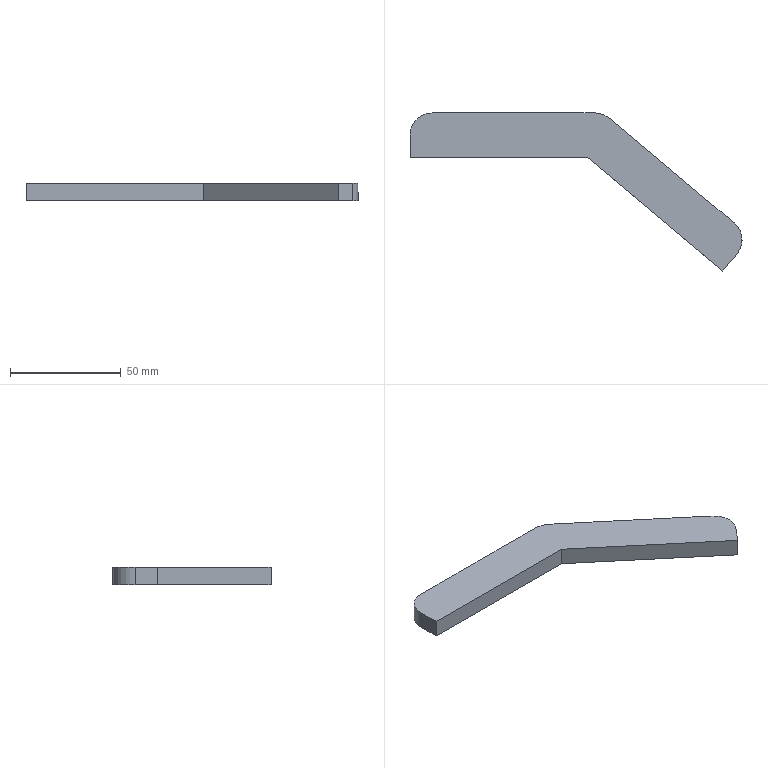Part | SolidWorks | features Extrusion 1, Fillet 1 | 1 solid | 11 faces | box 150.051 x 71.423 x 8 mm | volume 26409 mm3 | plane 8 | cylinder 3 | commonest cylinder face diameters 20 x3
STEP:
#1=CARTESIAN_POINT('',(0.,10.,8.));
#2=VERTEX_POINT('',#1);
#3=CARTESIAN_POINT('',(0.,0.,8.));
#4=VERTEX_POINT('',#3);
#5=CARTESIAN_POINT('',(0.,20.,8.));
#6=DIRECTION('',(0.,-1.,0.));
#7=VECTOR('',#6,1000.);
#8=LINE('',#5,#7);
#9=EDGE_CURVE('',#2,#4,#8,.T.);
#10=ORIENTED_EDGE('',*,*,#9,.F.);
#11=CARTESIAN_POINT('',(0.,10.,0.));
#12=VERTEX_POINT('',#11);
#13=CARTESIAN_POINT('',(0.,10.,8.));
#14=DIRECTION('',(0.,0.,-1.));
#15=VECTOR('',#14,1000.);
#16=LINE('',#13,#15);
#17=EDGE_CURVE('',#2,#12,#16,.T.);
#18=ORIENTED_EDGE('',*,*,#17,.T.);
#19=CARTESIAN_POINT('',(0.,0.,0.));
#20=VERTEX_POINT('',#19);
#21=CARTESIAN_POINT('',(0.,20.,0.));
#22=DIRECTION('',(0.,-1.,0.));
#23=VECTOR('',#22,1000.);
#24=LINE('',#21,#23);
#25=EDGE_CURVE('',#12,#20,#24,.T.);
#26=ORIENTED_EDGE('',*,*,#25,.T.);
#27=CARTESIAN_POINT('',(0.,0.,8.));
#28=DIRECTION('',(0.,0.,-1.));
#29=VECTOR('',#28,1000.);
#30=LINE('',#27,#29);
#31=EDGE_CURVE('',#4,#20,#30,.T.);
#32=ORIENTED_EDGE('',*,*,#31,.F.);
#33=EDGE_LOOP('',(#10,#18,#26,#32));
#34=FACE_OUTER_BOUND('',#33,.T.);
#35=CARTESIAN_POINT('',(0.,20.,8.));
#36=DIRECTION('',(1.,0.,0.));
#37=DIRECTION('',(0.,1.,0.));
#38=AXIS2_PLACEMENT_3D('',#35,#36,#37);
#39=PLANE('',#38);
#40=ADVANCED_FACE('',(#34),#39,.F.);
#41=CARTESIAN_POINT('',(80.,0.,0.));
#42=VERTEX_POINT('',#41);
#43=CARTESIAN_POINT('',(0.,0.,0.));
#44=DIRECTION('',(1.,0.,0.));
#45=VECTOR('',#44,1000.);
#46=LINE('',#43,#45);
#47=EDGE_CURVE('',#20,#42,#46,.T.);
#48=ORIENTED_EDGE('',*,*,#47,.T.);
#49=CARTESIAN_POINT('',(80.,0.,8.));
#50=VERTEX_POINT('',#49);
#51=CARTESIAN_POINT('',(80.,0.,8.));
#52=DIRECTION('',(0.,0.,-1.));
#53=VECTOR('',#52,1000.);
#54=LINE('',#51,#53);
#55=EDGE_CURVE('',#50,#42,#54,.T.);
#56=ORIENTED_EDGE('',*,*,#55,.F.);
#57=CARTESIAN_POINT('',(0.,0.,8.));
#58=DIRECTION('',(1.,0.,0.));
#59=VECTOR('',#58,1000.);
#60=LINE('',#57,#59);
#61=EDGE_CURVE('',#4,#50,#60,.T.);
#62=ORIENTED_EDGE('',*,*,#61,.F.);
#63=ORIENTED_EDGE('',*,*,#31,.T.);
#64=EDGE_LOOP('',(#48,#56,#62,#63));
#65=FACE_OUTER_BOUND('',#64,.T.);
#66=CARTESIAN_POINT('',(0.,0.,8.));
#67=DIRECTION('',(0.,1.,0.));
#68=DIRECTION('',(0.,0.,1.));
#69=AXIS2_PLACEMENT_3D('',#66,#67,#68);
#70=PLANE('',#69);
#71=ADVANCED_FACE('',(#65),#70,.F.);
#72=CARTESIAN_POINT('',(141.284,-51.423,0.));
#73=VERTEX_POINT('',#72);
#74=CARTESIAN_POINT('',(80.,0.,0.));
#75=DIRECTION('',(0.766,-0.6428,0.));
#76=VECTOR('',#75,1000.);
#77=LINE('',#74,#76);
#78=EDGE_CURVE('',#42,#73,#77,.T.);
#79=ORIENTED_EDGE('',*,*,#78,.T.);
#80=CARTESIAN_POINT('',(141.284,-51.423,8.));
#81=VERTEX_POINT('',#80);
#82=CARTESIAN_POINT('',(141.284,-51.423,8.));
#83=DIRECTION('',(0.,0.,-1.));
#84=VECTOR('',#83,1000.);
#85=LINE('',#82,#84);
#86=EDGE_CURVE('',#81,#73,#85,.T.);
#87=ORIENTED_EDGE('',*,*,#86,.F.);
#88=CARTESIAN_POINT('',(80.,0.,8.));
#89=DIRECTION('',(0.766,-0.6428,0.));
#90=VECTOR('',#89,1000.);
#91=LINE('',#88,#90);
#92=EDGE_CURVE('',#50,#81,#91,.T.);
#93=ORIENTED_EDGE('',*,*,#92,.F.);
#94=ORIENTED_EDGE('',*,*,#55,.T.);
#95=EDGE_LOOP('',(#79,#87,#93,#94));
#96=FACE_OUTER_BOUND('',#95,.T.);
#97=CARTESIAN_POINT('',(80.,0.,8.));
#98=DIRECTION('',(0.6428,0.766,0.));
#99=DIRECTION('',(-0.766,0.6428,0.));
#100=AXIS2_PLACEMENT_3D('',#97,#98,#99);
#101=PLANE('',#100);
#102=ADVANCED_FACE('',(#96),#101,.F.);
#103=CARTESIAN_POINT('',(147.711,-43.763,0.));
#104=VERTEX_POINT('',#103);
#105=CARTESIAN_POINT('',(141.284,-51.423,0.));
#106=DIRECTION('',(0.6428,0.766,0.));
#107=VECTOR('',#106,1000.);
#108=LINE('',#105,#107);
#109=EDGE_CURVE('',#73,#104,#108,.T.);
#110=ORIENTED_EDGE('',*,*,#109,.T.);
#111=CARTESIAN_POINT('',(147.711,-43.763,8.));
#112=VERTEX_POINT('',#111);
#113=CARTESIAN_POINT('',(147.711,-43.763,8.));
#114=DIRECTION('',(0.,0.,1.));
#115=VECTOR('',#114,1000.);
#116=LINE('',#113,#115);
#117=EDGE_CURVE('',#104,#112,#116,.T.);
#118=ORIENTED_EDGE('',*,*,#117,.T.);
#119=CARTESIAN_POINT('',(141.284,-51.423,8.));
#120=DIRECTION('',(0.6428,0.766,0.));
#121=VECTOR('',#120,1000.);
#122=LINE('',#119,#121);
#123=EDGE_CURVE('',#81,#112,#122,.T.);
#124=ORIENTED_EDGE('',*,*,#123,.F.);
#125=ORIENTED_EDGE('',*,*,#86,.T.);
#126=EDGE_LOOP('',(#110,#118,#124,#125));
#127=FACE_OUTER_BOUND('',#126,.T.);
#128=CARTESIAN_POINT('',(141.284,-51.423,8.));
#129=DIRECTION('',(-0.766,0.6428,0.));
#130=DIRECTION('',(-0.6428,-0.766,0.));
#131=AXIS2_PLACEMENT_3D('',#128,#129,#130);
#132=PLANE('',#131);
#133=ADVANCED_FACE('',(#127),#132,.F.);
#134=CARTESIAN_POINT('',(146.479,-29.674,0.));
#135=VERTEX_POINT('',#134);
#136=CARTESIAN_POINT('',(90.068,17.66,0.));
#137=VERTEX_POINT('',#136);
#138=CARTESIAN_POINT('',(154.139,-36.102,0.));
#139=DIRECTION('',(-0.766,0.6428,0.));
#140=VECTOR('',#139,1000.);
#141=LINE('',#138,#140);
#142=EDGE_CURVE('',#135,#137,#141,.T.);
#143=ORIENTED_EDGE('',*,*,#142,.T.);
#144=CARTESIAN_POINT('',(90.068,17.66,8.));
#145=VERTEX_POINT('',#144);
#146=CARTESIAN_POINT('',(90.068,17.66,8.));
#147=DIRECTION('',(0.,0.,1.));
#148=VECTOR('',#147,1000.);
#149=LINE('',#146,#148);
#150=EDGE_CURVE('',#137,#145,#149,.T.);
#151=ORIENTED_EDGE('',*,*,#150,.T.);
#152=CARTESIAN_POINT('',(146.479,-29.674,8.));
#153=VERTEX_POINT('',#152);
#154=CARTESIAN_POINT('',(154.139,-36.102,8.));
#155=DIRECTION('',(-0.766,0.6428,0.));
#156=VECTOR('',#155,1000.);
#157=LINE('',#154,#156);
#158=EDGE_CURVE('',#153,#145,#157,.T.);
#159=ORIENTED_EDGE('',*,*,#158,.F.);
#160=CARTESIAN_POINT('',(146.479,-29.674,8.));
#161=DIRECTION('',(0.,0.,-1.));
#162=VECTOR('',#161,1000.);
#163=LINE('',#160,#162);
#164=EDGE_CURVE('',#153,#135,#163,.T.);
#165=ORIENTED_EDGE('',*,*,#164,.T.);
#166=EDGE_LOOP('',(#143,#151,#159,#165));
#167=FACE_OUTER_BOUND('',#166,.T.);
#168=CARTESIAN_POINT('',(154.139,-36.102,8.));
#169=DIRECTION('',(-0.6428,-0.766,0.));
#170=DIRECTION('',(0.766,-0.6428,0.));
#171=AXIS2_PLACEMENT_3D('',#168,#169,#170);
#172=PLANE('',#171);
#173=ADVANCED_FACE('',(#167),#172,.F.);
#174=CARTESIAN_POINT('',(83.64,20.,8.));
#175=VERTEX_POINT('',#174);
#176=CARTESIAN_POINT('',(10.,20.,8.));
#177=VERTEX_POINT('',#176);
#178=CARTESIAN_POINT('',(87.279,20.,8.));
#179=DIRECTION('',(-1.,0.,0.));
#180=VECTOR('',#179,1000.);
#181=LINE('',#178,#180);
#182=EDGE_CURVE('',#175,#177,#181,.T.);
#183=ORIENTED_EDGE('',*,*,#182,.F.);
#184=CARTESIAN_POINT('',(83.64,20.,0.));
#185=VERTEX_POINT('',#184);
#186=CARTESIAN_POINT('',(83.64,20.,8.));
#187=DIRECTION('',(0.,0.,-1.));
#188=VECTOR('',#187,1000.);
#189=LINE('',#186,#188);
#190=EDGE_CURVE('',#175,#185,#189,.T.);
#191=ORIENTED_EDGE('',*,*,#190,.T.);
#192=CARTESIAN_POINT('',(10.,20.,0.));
#193=VERTEX_POINT('',#192);
#194=CARTESIAN_POINT('',(87.279,20.,0.));
#195=DIRECTION('',(-1.,0.,0.));
#196=VECTOR('',#195,1000.);
#197=LINE('',#194,#196);
#198=EDGE_CURVE('',#185,#193,#197,.T.);
#199=ORIENTED_EDGE('',*,*,#198,.T.);
#200=CARTESIAN_POINT('',(10.,20.,8.));
#201=DIRECTION('',(0.,0.,1.));
#202=VECTOR('',#201,1000.);
#203=LINE('',#200,#202);
#204=EDGE_CURVE('',#193,#177,#203,.T.);
#205=ORIENTED_EDGE('',*,*,#204,.T.);
#206=EDGE_LOOP('',(#183,#191,#199,#205));
#207=FACE_OUTER_BOUND('',#206,.T.);
#208=CARTESIAN_POINT('',(87.279,20.,8.));
#209=DIRECTION('',(0.,-1.,0.));
#210=DIRECTION('',(1.,0.,0.));
#211=AXIS2_PLACEMENT_3D('',#208,#209,#210);
#212=PLANE('',#211);
#213=ADVANCED_FACE('',(#207),#212,.F.);
#214=ORIENTED_EDGE('',*,*,#158,.T.);
#215=CARTESIAN_POINT('',(83.64,10.,8.));
#216=DIRECTION('',(0.,0.,1.));
#217=DIRECTION('',(1.,0.,0.));
#218=AXIS2_PLACEMENT_3D('',#215,#216,#217);
#219=CIRCLE('',#218,10.);
#220=EDGE_CURVE('',#145,#175,#219,.T.);
#221=ORIENTED_EDGE('',*,*,#220,.T.);
#222=ORIENTED_EDGE('',*,*,#182,.T.);
#223=CARTESIAN_POINT('',(10.,10.,8.));
#224=DIRECTION('',(0.,0.,1.));
#225=DIRECTION('',(1.,0.,0.));
#226=AXIS2_PLACEMENT_3D('',#223,#224,#225);
#227=CIRCLE('',#226,10.);
#228=EDGE_CURVE('',#177,#2,#227,.T.);
#229=ORIENTED_EDGE('',*,*,#228,.T.);
#230=ORIENTED_EDGE('',*,*,#9,.T.);
#231=ORIENTED_EDGE('',*,*,#61,.T.);
#232=ORIENTED_EDGE('',*,*,#92,.T.);
#233=ORIENTED_EDGE('',*,*,#123,.T.);
#234=CARTESIAN_POINT('',(140.051,-37.335,8.));
#235=DIRECTION('',(0.,0.,1.));
#236=DIRECTION('',(1.,0.,0.));
#237=AXIS2_PLACEMENT_3D('',#234,#235,#236);
#238=CIRCLE('',#237,10.);
#239=EDGE_CURVE('',#112,#153,#238,.T.);
#240=ORIENTED_EDGE('',*,*,#239,.T.);
#241=EDGE_LOOP('',(#214,#221,#222,#229,#230,#231,#232,#233,#240));
#242=FACE_OUTER_BOUND('',#241,.T.);
#243=CARTESIAN_POINT('',(0.,0.,8.));
#244=DIRECTION('',(0.,0.,1.));
#245=DIRECTION('',(1.,0.,0.));
#246=AXIS2_PLACEMENT_3D('',#243,#244,#245);
#247=PLANE('',#246);
#248=ADVANCED_FACE('',(#242),#247,.T.);
#249=ORIENTED_EDGE('',*,*,#198,.F.);
#250=CARTESIAN_POINT('',(83.64,10.,0.));
#251=DIRECTION('',(0.,0.,-1.));
#252=DIRECTION('',(1.,0.,0.));
#253=AXIS2_PLACEMENT_3D('',#250,#251,#252);
#254=CIRCLE('',#253,10.);
#255=EDGE_CURVE('',#185,#137,#254,.T.);
#256=ORIENTED_EDGE('',*,*,#255,.T.);
#257=ORIENTED_EDGE('',*,*,#142,.F.);
#258=CARTESIAN_POINT('',(140.051,-37.335,0.));
#259=DIRECTION('',(0.,0.,-1.));
#260=DIRECTION('',(1.,0.,0.));
#261=AXIS2_PLACEMENT_3D('',#258,#259,#260);
#262=CIRCLE('',#261,10.);
#263=EDGE_CURVE('',#135,#104,#262,.T.);
#264=ORIENTED_EDGE('',*,*,#263,.T.);
#265=ORIENTED_EDGE('',*,*,#109,.F.);
#266=ORIENTED_EDGE('',*,*,#78,.F.);
#267=ORIENTED_EDGE('',*,*,#47,.F.);
#268=ORIENTED_EDGE('',*,*,#25,.F.);
#269=CARTESIAN_POINT('',(10.,10.,0.));
#270=DIRECTION('',(0.,0.,-1.));
#271=DIRECTION('',(1.,0.,0.));
#272=AXIS2_PLACEMENT_3D('',#269,#270,#271);
#273=CIRCLE('',#272,10.);
#274=EDGE_CURVE('',#12,#193,#273,.T.);
#275=ORIENTED_EDGE('',*,*,#274,.T.);
#276=EDGE_LOOP('',(#249,#256,#257,#264,#265,#266,#267,#268,#275));
#277=FACE_OUTER_BOUND('',#276,.T.);
#278=CARTESIAN_POINT('',(0.,0.,0.));
#279=DIRECTION('',(0.,0.,1.));
#280=DIRECTION('',(1.,0.,0.));
#281=AXIS2_PLACEMENT_3D('',#278,#279,#280);
#282=PLANE('',#281);
#283=ADVANCED_FACE('',(#277),#282,.F.);
#284=ORIENTED_EDGE('',*,*,#220,.F.);
#285=ORIENTED_EDGE('',*,*,#150,.F.);
#286=ORIENTED_EDGE('',*,*,#255,.F.);
#287=ORIENTED_EDGE('',*,*,#190,.F.);
#288=EDGE_LOOP('',(#284,#285,#286,#287));
#289=FACE_OUTER_BOUND('',#288,.T.);
#290=CARTESIAN_POINT('',(83.64,10.,8.));
#291=DIRECTION('',(0.,0.,-1.));
#292=DIRECTION('',(-1.,0.,0.));
#293=AXIS2_PLACEMENT_3D('',#290,#291,#292);
#294=CYLINDRICAL_SURFACE('',#293,10.);
#295=ADVANCED_FACE('',(#289),#294,.T.);
#296=ORIENTED_EDGE('',*,*,#239,.F.);
#297=ORIENTED_EDGE('',*,*,#117,.F.);
#298=ORIENTED_EDGE('',*,*,#263,.F.);
#299=ORIENTED_EDGE('',*,*,#164,.F.);
#300=EDGE_LOOP('',(#296,#297,#298,#299));
#301=FACE_OUTER_BOUND('',#300,.T.);
#302=CARTESIAN_POINT('',(140.051,-37.335,8.));
#303=DIRECTION('',(0.,0.,-1.));
#304=DIRECTION('',(-1.,0.,0.));
#305=AXIS2_PLACEMENT_3D('',#302,#303,#304);
#306=CYLINDRICAL_SURFACE('',#305,10.);
#307=ADVANCED_FACE('',(#301),#306,.T.);
#308=ORIENTED_EDGE('',*,*,#228,.F.);
#309=ORIENTED_EDGE('',*,*,#204,.F.);
#310=ORIENTED_EDGE('',*,*,#274,.F.);
#311=ORIENTED_EDGE('',*,*,#17,.F.);
#312=EDGE_LOOP('',(#308,#309,#310,#311));
#313=FACE_OUTER_BOUND('',#312,.T.);
#314=CARTESIAN_POINT('',(10.,10.,8.));
#315=DIRECTION('',(0.,0.,-1.));
#316=DIRECTION('',(-1.,0.,0.));
#317=AXIS2_PLACEMENT_3D('',#314,#315,#316);
#318=CYLINDRICAL_SURFACE('',#317,10.);
#319=ADVANCED_FACE('',(#313),#318,.T.);
#320=CLOSED_SHELL('',(#40,#71,#102,#133,#173,#213,#248,#283,#295,#307,#319));
#321=MANIFOLD_SOLID_BREP('',#320);
#322=CARTESIAN_POINT('',(0.,0.,0.));
#323=DIRECTION('',(0.,0.,1.));
#324=DIRECTION('',(1.,0.,0.));
#325=AXIS2_PLACEMENT_3D('',#322,#323,#324);
#326=(LENGTH_UNIT()NAMED_UNIT(*)SI_UNIT(.MILLI.,.METRE.));
#327=UNCERTAINTY_MEASURE_WITH_UNIT(LENGTH_MEASURE(0.00001),#326,'','');
#328=(NAMED_UNIT(*)PLANE_ANGLE_UNIT()SI_UNIT($,.RADIAN.));
#329=(NAMED_UNIT(*)SI_UNIT($,.STERADIAN.)SOLID_ANGLE_UNIT());
#330=(GEOMETRIC_REPRESENTATION_CONTEXT(3)GLOBAL_UNCERTAINTY_ASSIGNED_CONTEXT((#327))GLOBAL_UNIT_ASSIGNED_CONTEXT((#326,#328,#329))REPRESENTATION_CONTEXT('',''));
#331=ADVANCED_BREP_SHAPE_REPRESENTATION('',(#321,#325),#330);